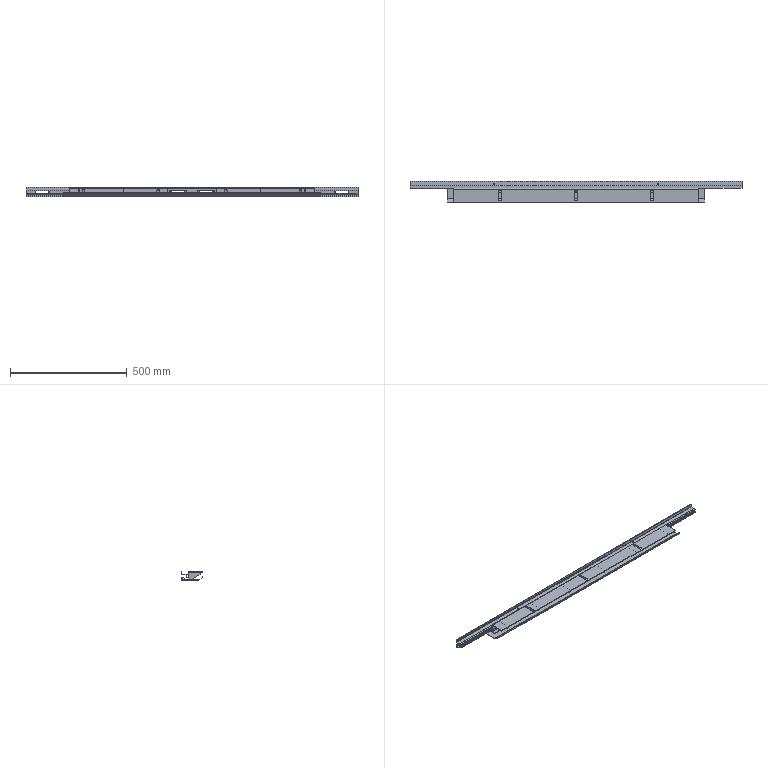Part | 9 solids | 263 faces | box 1420 x 92.321 x 40 mm | volume 717212 mm3 | plane 171 | cylinder 92 | commonest cylinder face diameters 9 x30 6 x25 10 x18 2 x9 12 x4 3 x2